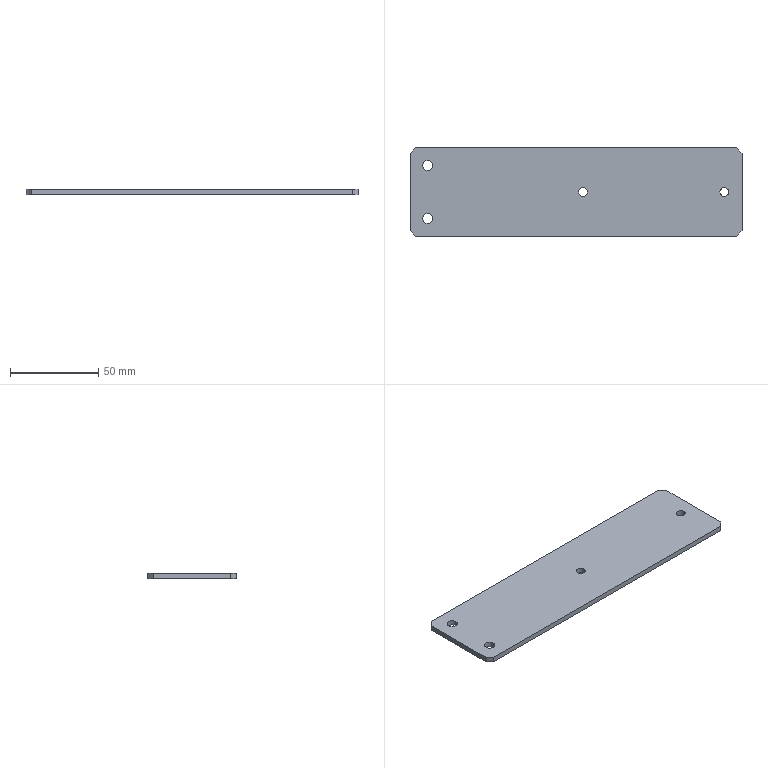Part | STEP file | J014-EBZ05-18-06-Part-1 | 1 solid | 18 faces | box 188 x 50 x 3 mm | volume 27870 mm3 | plane 10 | cylinder 8 | commonest cylinder face diameters 5 x4 5.8 x4
STEP:
#1=CARTESIAN_POINT('',(7.1,40.,3.));
#2=VERTEX_POINT('',#1);
#3=CARTESIAN_POINT('',(12.9,40.,3.));
#4=VERTEX_POINT('',#3);
#5=CARTESIAN_POINT('',(10.,40.,3.));
#6=DIRECTION('',(0.,0.,-1.));
#7=DIRECTION('',(1.,0.,0.));
#8=AXIS2_PLACEMENT_3D('',#5,#6,#7);
#9=CIRCLE('',#8,2.9);
#10=EDGE_CURVE('',#2,#4,#9,.T.);
#11=ORIENTED_EDGE('',*,*,#10,.F.);
#12=CARTESIAN_POINT('',(7.1,40.,0.));
#13=VERTEX_POINT('',#12);
#14=CARTESIAN_POINT('',(7.1,40.,3.));
#15=DIRECTION('',(0.,0.,-1.));
#16=VECTOR('',#15,1000.);
#17=LINE('',#14,#16);
#18=EDGE_CURVE('',#2,#13,#17,.T.);
#19=ORIENTED_EDGE('',*,*,#18,.T.);
#20=CARTESIAN_POINT('',(12.9,40.,0.));
#21=VERTEX_POINT('',#20);
#22=CARTESIAN_POINT('',(10.,40.,0.));
#23=DIRECTION('',(0.,0.,1.));
#24=DIRECTION('',(-1.,0.,0.));
#25=AXIS2_PLACEMENT_3D('',#22,#23,#24);
#26=CIRCLE('',#25,2.9);
#27=EDGE_CURVE('',#21,#13,#26,.T.);
#28=ORIENTED_EDGE('',*,*,#27,.F.);
#29=CARTESIAN_POINT('',(12.9,40.,3.));
#30=DIRECTION('',(0.,0.,-1.));
#31=VECTOR('',#30,1000.);
#32=LINE('',#29,#31);
#33=EDGE_CURVE('',#4,#21,#32,.T.);
#34=ORIENTED_EDGE('',*,*,#33,.F.);
#35=EDGE_LOOP('',(#11,#19,#28,#34));
#36=FACE_OUTER_BOUND('',#35,.T.);
#37=CARTESIAN_POINT('',(10.,40.,3.));
#38=DIRECTION('',(0.,0.,-1.));
#39=DIRECTION('',(1.,0.,0.));
#40=AXIS2_PLACEMENT_3D('',#37,#38,#39);
#41=CYLINDRICAL_SURFACE('',#40,2.9);
#42=ADVANCED_FACE('',(#36),#41,.F.);
#43=CARTESIAN_POINT('',(7.1,10.,3.));
#44=VERTEX_POINT('',#43);
#45=CARTESIAN_POINT('',(12.9,10.,3.));
#46=VERTEX_POINT('',#45);
#47=CARTESIAN_POINT('',(10.,10.,3.));
#48=DIRECTION('',(0.,0.,-1.));
#49=DIRECTION('',(1.,0.,0.));
#50=AXIS2_PLACEMENT_3D('',#47,#48,#49);
#51=CIRCLE('',#50,2.9);
#52=EDGE_CURVE('',#44,#46,#51,.T.);
#53=ORIENTED_EDGE('',*,*,#52,.F.);
#54=CARTESIAN_POINT('',(7.1,10.,0.));
#55=VERTEX_POINT('',#54);
#56=CARTESIAN_POINT('',(7.1,10.,3.));
#57=DIRECTION('',(0.,0.,-1.));
#58=VECTOR('',#57,1000.);
#59=LINE('',#56,#58);
#60=EDGE_CURVE('',#44,#55,#59,.T.);
#61=ORIENTED_EDGE('',*,*,#60,.T.);
#62=CARTESIAN_POINT('',(12.9,10.,0.));
#63=VERTEX_POINT('',#62);
#64=CARTESIAN_POINT('',(10.,10.,0.));
#65=DIRECTION('',(0.,0.,1.));
#66=DIRECTION('',(-1.,0.,0.));
#67=AXIS2_PLACEMENT_3D('',#64,#65,#66);
#68=CIRCLE('',#67,2.9);
#69=EDGE_CURVE('',#63,#55,#68,.T.);
#70=ORIENTED_EDGE('',*,*,#69,.F.);
#71=CARTESIAN_POINT('',(12.9,10.,3.));
#72=DIRECTION('',(0.,0.,-1.));
#73=VECTOR('',#72,1000.);
#74=LINE('',#71,#73);
#75=EDGE_CURVE('',#46,#63,#74,.T.);
#76=ORIENTED_EDGE('',*,*,#75,.F.);
#77=EDGE_LOOP('',(#53,#61,#70,#76));
#78=FACE_OUTER_BOUND('',#77,.T.);
#79=CARTESIAN_POINT('',(10.,10.,3.));
#80=DIRECTION('',(0.,0.,-1.));
#81=DIRECTION('',(1.,0.,0.));
#82=AXIS2_PLACEMENT_3D('',#79,#80,#81);
#83=CYLINDRICAL_SURFACE('',#82,2.9);
#84=ADVANCED_FACE('',(#78),#83,.F.);
#85=CARTESIAN_POINT('',(180.5,25.,0.));
#86=VERTEX_POINT('',#85);
#87=CARTESIAN_POINT('',(175.5,25.,0.));
#88=VERTEX_POINT('',#87);
#89=CARTESIAN_POINT('',(178.,25.,0.));
#90=DIRECTION('',(0.,0.,1.));
#91=DIRECTION('',(-1.,0.,0.));
#92=AXIS2_PLACEMENT_3D('',#89,#90,#91);
#93=CIRCLE('',#92,2.5);
#94=EDGE_CURVE('',#86,#88,#93,.T.);
#95=ORIENTED_EDGE('',*,*,#94,.F.);
#96=CARTESIAN_POINT('',(180.5,25.,3.));
#97=VERTEX_POINT('',#96);
#98=CARTESIAN_POINT('',(180.5,25.,0.));
#99=DIRECTION('',(0.,0.,1.));
#100=VECTOR('',#99,1000.);
#101=LINE('',#98,#100);
#102=EDGE_CURVE('',#86,#97,#101,.T.);
#103=ORIENTED_EDGE('',*,*,#102,.T.);
#104=CARTESIAN_POINT('',(175.5,25.,3.));
#105=VERTEX_POINT('',#104);
#106=CARTESIAN_POINT('',(178.,25.,3.));
#107=DIRECTION('',(0.,0.,-1.));
#108=DIRECTION('',(1.,0.,0.));
#109=AXIS2_PLACEMENT_3D('',#106,#107,#108);
#110=CIRCLE('',#109,2.5);
#111=EDGE_CURVE('',#105,#97,#110,.T.);
#112=ORIENTED_EDGE('',*,*,#111,.F.);
#113=CARTESIAN_POINT('',(175.5,25.,0.));
#114=DIRECTION('',(0.,0.,1.));
#115=VECTOR('',#114,1000.);
#116=LINE('',#113,#115);
#117=EDGE_CURVE('',#88,#105,#116,.T.);
#118=ORIENTED_EDGE('',*,*,#117,.F.);
#119=EDGE_LOOP('',(#95,#103,#112,#118));
#120=FACE_OUTER_BOUND('',#119,.T.);
#121=CARTESIAN_POINT('',(178.,25.,0.));
#122=DIRECTION('',(0.,0.,1.));
#123=DIRECTION('',(-1.,0.,0.));
#124=AXIS2_PLACEMENT_3D('',#121,#122,#123);
#125=CYLINDRICAL_SURFACE('',#124,2.5);
#126=ADVANCED_FACE('',(#120),#125,.F.);
#127=CARTESIAN_POINT('',(100.5,25.,0.));
#128=VERTEX_POINT('',#127);
#129=CARTESIAN_POINT('',(95.5,25.,0.));
#130=VERTEX_POINT('',#129);
#131=CARTESIAN_POINT('',(98.,25.,0.));
#132=DIRECTION('',(0.,0.,1.));
#133=DIRECTION('',(-1.,0.,0.));
#134=AXIS2_PLACEMENT_3D('',#131,#132,#133);
#135=CIRCLE('',#134,2.5);
#136=EDGE_CURVE('',#128,#130,#135,.T.);
#137=ORIENTED_EDGE('',*,*,#136,.F.);
#138=CARTESIAN_POINT('',(100.5,25.,3.));
#139=VERTEX_POINT('',#138);
#140=CARTESIAN_POINT('',(100.5,25.,0.));
#141=DIRECTION('',(0.,0.,1.));
#142=VECTOR('',#141,1000.);
#143=LINE('',#140,#142);
#144=EDGE_CURVE('',#128,#139,#143,.T.);
#145=ORIENTED_EDGE('',*,*,#144,.T.);
#146=CARTESIAN_POINT('',(95.5,25.,3.));
#147=VERTEX_POINT('',#146);
#148=CARTESIAN_POINT('',(98.,25.,3.));
#149=DIRECTION('',(0.,0.,-1.));
#150=DIRECTION('',(1.,0.,0.));
#151=AXIS2_PLACEMENT_3D('',#148,#149,#150);
#152=CIRCLE('',#151,2.5);
#153=EDGE_CURVE('',#147,#139,#152,.T.);
#154=ORIENTED_EDGE('',*,*,#153,.F.);
#155=CARTESIAN_POINT('',(95.5,25.,0.));
#156=DIRECTION('',(0.,0.,1.));
#157=VECTOR('',#156,1000.);
#158=LINE('',#155,#157);
#159=EDGE_CURVE('',#130,#147,#158,.T.);
#160=ORIENTED_EDGE('',*,*,#159,.F.);
#161=EDGE_LOOP('',(#137,#145,#154,#160));
#162=FACE_OUTER_BOUND('',#161,.T.);
#163=CARTESIAN_POINT('',(98.,25.,0.));
#164=DIRECTION('',(0.,0.,1.));
#165=DIRECTION('',(-1.,0.,0.));
#166=AXIS2_PLACEMENT_3D('',#163,#164,#165);
#167=CYLINDRICAL_SURFACE('',#166,2.5);
#168=ADVANCED_FACE('',(#162),#167,.F.);
#169=CARTESIAN_POINT('',(185.,0.,0.));
#170=VERTEX_POINT('',#169);
#171=CARTESIAN_POINT('',(3.,0.,0.));
#172=VERTEX_POINT('',#171);
#173=CARTESIAN_POINT('',(94.,0.,0.));
#174=DIRECTION('',(-1.,0.,0.));
#175=VECTOR('',#174,1000.);
#176=LINE('',#173,#175);
#177=EDGE_CURVE('',#170,#172,#176,.T.);
#178=ORIENTED_EDGE('',*,*,#177,.F.);
#179=CARTESIAN_POINT('',(185.,0.,3.));
#180=VERTEX_POINT('',#179);
#181=CARTESIAN_POINT('',(185.,0.,1.5));
#182=DIRECTION('',(0.,0.,1.));
#183=VECTOR('',#182,1000.);
#184=LINE('',#181,#183);
#185=EDGE_CURVE('',#170,#180,#184,.T.);
#186=ORIENTED_EDGE('',*,*,#185,.T.);
#187=CARTESIAN_POINT('',(3.,0.,3.));
#188=VERTEX_POINT('',#187);
#189=CARTESIAN_POINT('',(94.,0.,3.));
#190=DIRECTION('',(1.,0.,0.));
#191=VECTOR('',#190,1000.);
#192=LINE('',#189,#191);
#193=EDGE_CURVE('',#188,#180,#192,.T.);
#194=ORIENTED_EDGE('',*,*,#193,.F.);
#195=CARTESIAN_POINT('',(3.,0.,1.5));
#196=DIRECTION('',(0.,0.,-1.));
#197=VECTOR('',#196,1000.);
#198=LINE('',#195,#197);
#199=EDGE_CURVE('',#188,#172,#198,.T.);
#200=ORIENTED_EDGE('',*,*,#199,.T.);
#201=EDGE_LOOP('',(#178,#186,#194,#200));
#202=FACE_OUTER_BOUND('',#201,.T.);
#203=CARTESIAN_POINT('',(94.,0.,1.5));
#204=DIRECTION('',(0.,-1.,0.));
#205=DIRECTION('',(1.,0.,0.));
#206=AXIS2_PLACEMENT_3D('',#203,#204,#205);
#207=PLANE('',#206);
#208=ADVANCED_FACE('',(#202),#207,.T.);
#209=ORIENTED_EDGE('',*,*,#27,.T.);
#210=CARTESIAN_POINT('',(10.,40.,0.));
#211=DIRECTION('',(0.,0.,1.));
#212=DIRECTION('',(-1.,0.,0.));
#213=AXIS2_PLACEMENT_3D('',#210,#211,#212);
#214=CIRCLE('',#213,2.9);
#215=EDGE_CURVE('',#13,#21,#214,.T.);
#216=ORIENTED_EDGE('',*,*,#215,.T.);
#217=EDGE_LOOP('',(#209,#216));
#218=FACE_BOUND('',#217,.T.);
#219=ORIENTED_EDGE('',*,*,#69,.T.);
#220=CARTESIAN_POINT('',(10.,10.,0.));
#221=DIRECTION('',(0.,0.,1.));
#222=DIRECTION('',(-1.,0.,0.));
#223=AXIS2_PLACEMENT_3D('',#220,#221,#222);
#224=CIRCLE('',#223,2.9);
#225=EDGE_CURVE('',#55,#63,#224,.T.);
#226=ORIENTED_EDGE('',*,*,#225,.T.);
#227=EDGE_LOOP('',(#219,#226));
#228=FACE_BOUND('',#227,.T.);
#229=CARTESIAN_POINT('',(178.,25.,0.));
#230=DIRECTION('',(0.,0.,1.));
#231=DIRECTION('',(-1.,0.,0.));
#232=AXIS2_PLACEMENT_3D('',#229,#230,#231);
#233=CIRCLE('',#232,2.5);
#234=EDGE_CURVE('',#88,#86,#233,.T.);
#235=ORIENTED_EDGE('',*,*,#234,.T.);
#236=ORIENTED_EDGE('',*,*,#94,.T.);
#237=EDGE_LOOP('',(#235,#236));
#238=FACE_BOUND('',#237,.T.);
#239=CARTESIAN_POINT('',(98.,25.,0.));
#240=DIRECTION('',(0.,0.,1.));
#241=DIRECTION('',(-1.,0.,0.));
#242=AXIS2_PLACEMENT_3D('',#239,#240,#241);
#243=CIRCLE('',#242,2.5);
#244=EDGE_CURVE('',#130,#128,#243,.T.);
#245=ORIENTED_EDGE('',*,*,#244,.T.);
#246=ORIENTED_EDGE('',*,*,#136,.T.);
#247=EDGE_LOOP('',(#245,#246));
#248=FACE_BOUND('',#247,.T.);
#249=CARTESIAN_POINT('',(3.,50.,0.));
#250=VERTEX_POINT('',#249);
#251=CARTESIAN_POINT('',(185.,50.,0.));
#252=VERTEX_POINT('',#251);
#253=CARTESIAN_POINT('',(94.,50.,0.));
#254=DIRECTION('',(1.,0.,0.));
#255=VECTOR('',#254,1000.);
#256=LINE('',#253,#255);
#257=EDGE_CURVE('',#250,#252,#256,.T.);
#258=ORIENTED_EDGE('',*,*,#257,.T.);
#259=CARTESIAN_POINT('',(188.,47.,0.));
#260=VERTEX_POINT('',#259);
#261=CARTESIAN_POINT('',(139.5,95.5,0.));
#262=DIRECTION('',(0.7071,-0.7071,0.));
#263=VECTOR('',#262,1000.);
#264=LINE('',#261,#263);
#265=EDGE_CURVE('',#252,#260,#264,.T.);
#266=ORIENTED_EDGE('',*,*,#265,.T.);
#267=CARTESIAN_POINT('',(188.,3.,0.));
#268=VERTEX_POINT('',#267);
#269=CARTESIAN_POINT('',(188.,50.,0.));
#270=DIRECTION('',(0.,-1.,0.));
#271=VECTOR('',#270,1000.);
#272=LINE('',#269,#271);
#273=EDGE_CURVE('',#260,#268,#272,.T.);
#274=ORIENTED_EDGE('',*,*,#273,.T.);
#275=CARTESIAN_POINT('',(164.5,-20.5,0.));
#276=DIRECTION('',(-0.7071,-0.7071,0.));
#277=VECTOR('',#276,1000.);
#278=LINE('',#275,#277);
#279=EDGE_CURVE('',#268,#170,#278,.T.);
#280=ORIENTED_EDGE('',*,*,#279,.T.);
#281=ORIENTED_EDGE('',*,*,#177,.T.);
#282=CARTESIAN_POINT('',(0.,3.,0.));
#283=VERTEX_POINT('',#282);
#284=CARTESIAN_POINT('',(23.5,-20.5,0.));
#285=DIRECTION('',(-0.7071,0.7071,0.));
#286=VECTOR('',#285,1000.);
#287=LINE('',#284,#286);
#288=EDGE_CURVE('',#172,#283,#287,.T.);
#289=ORIENTED_EDGE('',*,*,#288,.T.);
#290=CARTESIAN_POINT('',(0.,47.,0.));
#291=VERTEX_POINT('',#290);
#292=CARTESIAN_POINT('',(0.,50.,0.));
#293=DIRECTION('',(0.,-1.,0.));
#294=VECTOR('',#293,1000.);
#295=LINE('',#292,#294);
#296=EDGE_CURVE('',#291,#283,#295,.T.);
#297=ORIENTED_EDGE('',*,*,#296,.F.);
#298=CARTESIAN_POINT('',(48.5,95.5,0.));
#299=DIRECTION('',(0.7071,0.7071,0.));
#300=VECTOR('',#299,1000.);
#301=LINE('',#298,#300);
#302=EDGE_CURVE('',#291,#250,#301,.T.);
#303=ORIENTED_EDGE('',*,*,#302,.T.);
#304=EDGE_LOOP('',(#258,#266,#274,#280,#281,#289,#297,#303));
#305=FACE_OUTER_BOUND('',#304,.T.);
#306=CARTESIAN_POINT('',(94.,50.,0.));
#307=DIRECTION('',(0.,0.,-1.));
#308=DIRECTION('',(0.,1.,0.));
#309=AXIS2_PLACEMENT_3D('',#306,#307,#308);
#310=PLANE('',#309);
#311=ADVANCED_FACE('',(#218,#228,#238,#248,#305),#310,.T.);
#312=ORIENTED_EDGE('',*,*,#296,.T.);
#313=CARTESIAN_POINT('',(0.,3.,3.));
#314=VERTEX_POINT('',#313);
#315=CARTESIAN_POINT('',(0.,3.,1.5));
#316=DIRECTION('',(0.,0.,1.));
#317=VECTOR('',#316,1000.);
#318=LINE('',#315,#317);
#319=EDGE_CURVE('',#283,#314,#318,.T.);
#320=ORIENTED_EDGE('',*,*,#319,.T.);
#321=CARTESIAN_POINT('',(0.,47.,3.));
#322=VERTEX_POINT('',#321);
#323=CARTESIAN_POINT('',(0.,50.,3.));
#324=DIRECTION('',(0.,-1.,0.));
#325=VECTOR('',#324,1000.);
#326=LINE('',#323,#325);
#327=EDGE_CURVE('',#322,#314,#326,.T.);
#328=ORIENTED_EDGE('',*,*,#327,.F.);
#329=CARTESIAN_POINT('',(0.,47.,1.5));
#330=DIRECTION('',(0.,0.,-1.));
#331=VECTOR('',#330,1000.);
#332=LINE('',#329,#331);
#333=EDGE_CURVE('',#322,#291,#332,.T.);
#334=ORIENTED_EDGE('',*,*,#333,.T.);
#335=EDGE_LOOP('',(#312,#320,#328,#334));
#336=FACE_OUTER_BOUND('',#335,.T.);
#337=CARTESIAN_POINT('',(0.,50.,1.5));
#338=DIRECTION('',(-1.,0.,0.));
#339=DIRECTION('',(0.,-1.,0.));
#340=AXIS2_PLACEMENT_3D('',#337,#338,#339);
#341=PLANE('',#340);
#342=ADVANCED_FACE('',(#336),#341,.T.);
#343=CARTESIAN_POINT('',(10.,40.,3.));
#344=DIRECTION('',(0.,0.,-1.));
#345=DIRECTION('',(1.,0.,0.));
#346=AXIS2_PLACEMENT_3D('',#343,#344,#345);
#347=CIRCLE('',#346,2.9);
#348=EDGE_CURVE('',#4,#2,#347,.T.);
#349=ORIENTED_EDGE('',*,*,#348,.T.);
#350=ORIENTED_EDGE('',*,*,#10,.T.);
#351=EDGE_LOOP('',(#349,#350));
#352=FACE_BOUND('',#351,.T.);
#353=CARTESIAN_POINT('',(10.,10.,3.));
#354=DIRECTION('',(0.,0.,-1.));
#355=DIRECTION('',(1.,0.,0.));
#356=AXIS2_PLACEMENT_3D('',#353,#354,#355);
#357=CIRCLE('',#356,2.9);
#358=EDGE_CURVE('',#46,#44,#357,.T.);
#359=ORIENTED_EDGE('',*,*,#358,.T.);
#360=ORIENTED_EDGE('',*,*,#52,.T.);
#361=EDGE_LOOP('',(#359,#360));
#362=FACE_BOUND('',#361,.T.);
#363=ORIENTED_EDGE('',*,*,#111,.T.);
#364=CARTESIAN_POINT('',(178.,25.,3.));
#365=DIRECTION('',(0.,0.,-1.));
#366=DIRECTION('',(1.,0.,0.));
#367=AXIS2_PLACEMENT_3D('',#364,#365,#366);
#368=CIRCLE('',#367,2.5);
#369=EDGE_CURVE('',#97,#105,#368,.T.);
#370=ORIENTED_EDGE('',*,*,#369,.T.);
#371=EDGE_LOOP('',(#363,#370));
#372=FACE_BOUND('',#371,.T.);
#373=ORIENTED_EDGE('',*,*,#153,.T.);
#374=CARTESIAN_POINT('',(98.,25.,3.));
#375=DIRECTION('',(0.,0.,-1.));
#376=DIRECTION('',(1.,0.,0.));
#377=AXIS2_PLACEMENT_3D('',#374,#375,#376);
#378=CIRCLE('',#377,2.5);
#379=EDGE_CURVE('',#139,#147,#378,.T.);
#380=ORIENTED_EDGE('',*,*,#379,.T.);
#381=EDGE_LOOP('',(#373,#380));
#382=FACE_BOUND('',#381,.T.);
#383=CARTESIAN_POINT('',(188.,47.,3.));
#384=VERTEX_POINT('',#383);
#385=CARTESIAN_POINT('',(188.,3.,3.));
#386=VERTEX_POINT('',#385);
#387=CARTESIAN_POINT('',(188.,50.,3.));
#388=DIRECTION('',(0.,-1.,0.));
#389=VECTOR('',#388,1000.);
#390=LINE('',#387,#389);
#391=EDGE_CURVE('',#384,#386,#390,.T.);
#392=ORIENTED_EDGE('',*,*,#391,.F.);
#393=CARTESIAN_POINT('',(185.,50.,3.));
#394=VERTEX_POINT('',#393);
#395=CARTESIAN_POINT('',(139.5,95.5,3.));
#396=DIRECTION('',(-0.7071,0.7071,0.));
#397=VECTOR('',#396,1000.);
#398=LINE('',#395,#397);
#399=EDGE_CURVE('',#384,#394,#398,.T.);
#400=ORIENTED_EDGE('',*,*,#399,.T.);
#401=CARTESIAN_POINT('',(3.,50.,3.));
#402=VERTEX_POINT('',#401);
#403=CARTESIAN_POINT('',(94.,50.,3.));
#404=DIRECTION('',(-1.,0.,0.));
#405=VECTOR('',#404,1000.);
#406=LINE('',#403,#405);
#407=EDGE_CURVE('',#394,#402,#406,.T.);
#408=ORIENTED_EDGE('',*,*,#407,.T.);
#409=CARTESIAN_POINT('',(48.5,95.5,3.));
#410=DIRECTION('',(-0.7071,-0.7071,0.));
#411=VECTOR('',#410,1000.);
#412=LINE('',#409,#411);
#413=EDGE_CURVE('',#402,#322,#412,.T.);
#414=ORIENTED_EDGE('',*,*,#413,.T.);
#415=ORIENTED_EDGE('',*,*,#327,.T.);
#416=CARTESIAN_POINT('',(23.5,-20.5,3.));
#417=DIRECTION('',(0.7071,-0.7071,0.));
#418=VECTOR('',#417,1000.);
#419=LINE('',#416,#418);
#420=EDGE_CURVE('',#314,#188,#419,.T.);
#421=ORIENTED_EDGE('',*,*,#420,.T.);
#422=ORIENTED_EDGE('',*,*,#193,.T.);
#423=CARTESIAN_POINT('',(164.5,-20.5,3.));
#424=DIRECTION('',(0.7071,0.7071,0.));
#425=VECTOR('',#424,1000.);
#426=LINE('',#423,#425);
#427=EDGE_CURVE('',#180,#386,#426,.T.);
#428=ORIENTED_EDGE('',*,*,#427,.T.);
#429=EDGE_LOOP('',(#392,#400,#408,#414,#415,#421,#422,#428));
#430=FACE_OUTER_BOUND('',#429,.T.);
#431=CARTESIAN_POINT('',(94.,50.,3.));
#432=DIRECTION('',(0.,0.,1.));
#433=DIRECTION('',(0.,-1.,0.));
#434=AXIS2_PLACEMENT_3D('',#431,#432,#433);
#435=PLANE('',#434);
#436=ADVANCED_FACE('',(#352,#362,#372,#382,#430),#435,.T.);
#437=ORIENTED_EDGE('',*,*,#407,.F.);
#438=CARTESIAN_POINT('',(185.,50.,1.5));
#439=DIRECTION('',(0.,0.,-1.));
#440=VECTOR('',#439,1000.);
#441=LINE('',#438,#440);
#442=EDGE_CURVE('',#394,#252,#441,.T.);
#443=ORIENTED_EDGE('',*,*,#442,.T.);
#444=ORIENTED_EDGE('',*,*,#257,.F.);
#445=CARTESIAN_POINT('',(3.,50.,1.5));
#446=DIRECTION('',(0.,0.,1.));
#447=VECTOR('',#446,1000.);
#448=LINE('',#445,#447);
#449=EDGE_CURVE('',#250,#402,#448,.T.);
#450=ORIENTED_EDGE('',*,*,#449,.T.);
#451=EDGE_LOOP('',(#437,#443,#444,#450));
#452=FACE_OUTER_BOUND('',#451,.T.);
#453=CARTESIAN_POINT('',(94.,50.,1.5));
#454=DIRECTION('',(0.,1.,0.));
#455=DIRECTION('',(-1.,0.,0.));
#456=AXIS2_PLACEMENT_3D('',#453,#454,#455);
#457=PLANE('',#456);
#458=ADVANCED_FACE('',(#452),#457,.T.);
#459=ORIENTED_EDGE('',*,*,#273,.F.);
#460=CARTESIAN_POINT('',(188.,47.,1.5));
#461=DIRECTION('',(0.,0.,1.));
#462=VECTOR('',#461,1000.);
#463=LINE('',#460,#462);
#464=EDGE_CURVE('',#260,#384,#463,.T.);
#465=ORIENTED_EDGE('',*,*,#464,.T.);
#466=ORIENTED_EDGE('',*,*,#391,.T.);
#467=CARTESIAN_POINT('',(188.,3.,1.5));
#468=DIRECTION('',(0.,0.,-1.));
#469=VECTOR('',#468,1000.);
#470=LINE('',#467,#469);
#471=EDGE_CURVE('',#386,#268,#470,.T.);
#472=ORIENTED_EDGE('',*,*,#471,.T.);
#473=EDGE_LOOP('',(#459,#465,#466,#472));
#474=FACE_OUTER_BOUND('',#473,.T.);
#475=CARTESIAN_POINT('',(188.,50.,1.5));
#476=DIRECTION('',(1.,0.,0.));
#477=DIRECTION('',(0.,1.,0.));
#478=AXIS2_PLACEMENT_3D('',#475,#476,#477);
#479=PLANE('',#478);
#480=ADVANCED_FACE('',(#474),#479,.T.);
#481=ORIENTED_EDGE('',*,*,#144,.F.);
#482=ORIENTED_EDGE('',*,*,#244,.F.);
#483=ORIENTED_EDGE('',*,*,#159,.T.);
#484=ORIENTED_EDGE('',*,*,#379,.F.);
#485=EDGE_LOOP('',(#481,#482,#483,#484));
#486=FACE_OUTER_BOUND('',#485,.T.);
#487=CARTESIAN_POINT('',(98.,25.,0.));
#488=DIRECTION('',(0.,0.,1.));
#489=DIRECTION('',(-1.,0.,0.));
#490=AXIS2_PLACEMENT_3D('',#487,#488,#489);
#491=CYLINDRICAL_SURFACE('',#490,2.5);
#492=ADVANCED_FACE('',(#486),#491,.F.);
#493=ORIENTED_EDGE('',*,*,#102,.F.);
#494=ORIENTED_EDGE('',*,*,#234,.F.);
#495=ORIENTED_EDGE('',*,*,#117,.T.);
#496=ORIENTED_EDGE('',*,*,#369,.F.);
#497=EDGE_LOOP('',(#493,#494,#495,#496));
#498=FACE_OUTER_BOUND('',#497,.T.);
#499=CARTESIAN_POINT('',(178.,25.,0.));
#500=DIRECTION('',(0.,0.,1.));
#501=DIRECTION('',(-1.,0.,0.));
#502=AXIS2_PLACEMENT_3D('',#499,#500,#501);
#503=CYLINDRICAL_SURFACE('',#502,2.5);
#504=ADVANCED_FACE('',(#498),#503,.F.);
#505=ORIENTED_EDGE('',*,*,#265,.F.);
#506=ORIENTED_EDGE('',*,*,#442,.F.);
#507=ORIENTED_EDGE('',*,*,#399,.F.);
#508=ORIENTED_EDGE('',*,*,#464,.F.);
#509=EDGE_LOOP('',(#505,#506,#507,#508));
#510=FACE_OUTER_BOUND('',#509,.T.);
#511=CARTESIAN_POINT('',(188.,47.,1.5));
#512=DIRECTION('',(-0.7071,-0.7071,0.));
#513=DIRECTION('',(0.,0.,1.));
#514=AXIS2_PLACEMENT_3D('',#511,#512,#513);
#515=PLANE('',#514);
#516=ADVANCED_FACE('',(#510),#515,.F.);
#517=ORIENTED_EDGE('',*,*,#427,.F.);
#518=ORIENTED_EDGE('',*,*,#185,.F.);
#519=ORIENTED_EDGE('',*,*,#279,.F.);
#520=ORIENTED_EDGE('',*,*,#471,.F.);
#521=EDGE_LOOP('',(#517,#518,#519,#520));
#522=FACE_OUTER_BOUND('',#521,.T.);
#523=CARTESIAN_POINT('',(188.,3.,1.5));
#524=DIRECTION('',(-0.7071,0.7071,0.));
#525=DIRECTION('',(0.,0.,-1.));
#526=AXIS2_PLACEMENT_3D('',#523,#524,#525);
#527=PLANE('',#526);
#528=ADVANCED_FACE('',(#522),#527,.F.);
#529=ORIENTED_EDGE('',*,*,#288,.F.);
#530=ORIENTED_EDGE('',*,*,#199,.F.);
#531=ORIENTED_EDGE('',*,*,#420,.F.);
#532=ORIENTED_EDGE('',*,*,#319,.F.);
#533=EDGE_LOOP('',(#529,#530,#531,#532));
#534=FACE_OUTER_BOUND('',#533,.T.);
#535=CARTESIAN_POINT('',(0.,3.,1.5));
#536=DIRECTION('',(0.7071,0.7071,0.));
#537=DIRECTION('',(0.,0.,1.));
#538=AXIS2_PLACEMENT_3D('',#535,#536,#537);
#539=PLANE('',#538);
#540=ADVANCED_FACE('',(#534),#539,.F.);
#541=ORIENTED_EDGE('',*,*,#413,.F.);
#542=ORIENTED_EDGE('',*,*,#449,.F.);
#543=ORIENTED_EDGE('',*,*,#302,.F.);
#544=ORIENTED_EDGE('',*,*,#333,.F.);
#545=EDGE_LOOP('',(#541,#542,#543,#544));
#546=FACE_OUTER_BOUND('',#545,.T.);
#547=CARTESIAN_POINT('',(0.,47.,1.5));
#548=DIRECTION('',(0.7071,-0.7071,0.));
#549=DIRECTION('',(0.,0.,-1.));
#550=AXIS2_PLACEMENT_3D('',#547,#548,#549);
#551=PLANE('',#550);
#552=ADVANCED_FACE('',(#546),#551,.F.);
#553=ORIENTED_EDGE('',*,*,#60,.F.);
#554=ORIENTED_EDGE('',*,*,#358,.F.);
#555=ORIENTED_EDGE('',*,*,#75,.T.);
#556=ORIENTED_EDGE('',*,*,#225,.F.);
#557=EDGE_LOOP('',(#553,#554,#555,#556));
#558=FACE_OUTER_BOUND('',#557,.T.);
#559=CARTESIAN_POINT('',(10.,10.,3.));
#560=DIRECTION('',(0.,0.,-1.));
#561=DIRECTION('',(1.,0.,0.));
#562=AXIS2_PLACEMENT_3D('',#559,#560,#561);
#563=CYLINDRICAL_SURFACE('',#562,2.9);
#564=ADVANCED_FACE('',(#558),#563,.F.);
#565=ORIENTED_EDGE('',*,*,#18,.F.);
#566=ORIENTED_EDGE('',*,*,#348,.F.);
#567=ORIENTED_EDGE('',*,*,#33,.T.);
#568=ORIENTED_EDGE('',*,*,#215,.F.);
#569=EDGE_LOOP('',(#565,#566,#567,#568));
#570=FACE_OUTER_BOUND('',#569,.T.);
#571=CARTESIAN_POINT('',(10.,40.,3.));
#572=DIRECTION('',(0.,0.,-1.));
#573=DIRECTION('',(1.,0.,0.));
#574=AXIS2_PLACEMENT_3D('',#571,#572,#573);
#575=CYLINDRICAL_SURFACE('',#574,2.9);
#576=ADVANCED_FACE('',(#570),#575,.F.);
#577=CLOSED_SHELL('',(#42,#84,#126,#168,#208,#311,#342,#436,#458,#480,#492,#504,#516,#528,#540,#552,#564,#576));
#578=MANIFOLD_SOLID_BREP('',#577);
#579=CARTESIAN_POINT('',(0.,0.,0.));
#580=DIRECTION('',(0.,0.,1.));
#581=DIRECTION('',(1.,0.,0.));
#582=AXIS2_PLACEMENT_3D('',#579,#580,#581);
#583=(LENGTH_UNIT()NAMED_UNIT(*)SI_UNIT(.MILLI.,.METRE.));
#584=UNCERTAINTY_MEASURE_WITH_UNIT(LENGTH_MEASURE(0.00001),#583,'','');
#585=(NAMED_UNIT(*)PLANE_ANGLE_UNIT()SI_UNIT($,.RADIAN.));
#586=(NAMED_UNIT(*)SI_UNIT($,.STERADIAN.)SOLID_ANGLE_UNIT());
#587=(GEOMETRIC_REPRESENTATION_CONTEXT(3)GLOBAL_UNCERTAINTY_ASSIGNED_CONTEXT((#584))GLOBAL_UNIT_ASSIGNED_CONTEXT((#583,#585,#586))REPRESENTATION_CONTEXT('',''));
#588=ADVANCED_BREP_SHAPE_REPRESENTATION('',(#578,#582),#587);